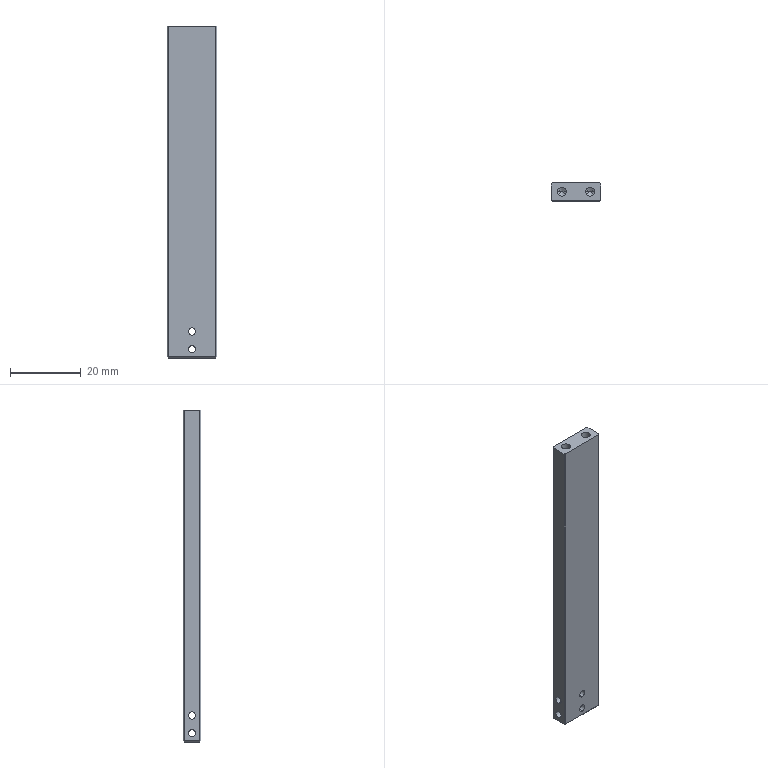Part | STEP file | Stopper bar | 1 solid | 42 faces | box 14 x 5 x 94 mm | volume 6342 mm3 | cylinder 20 | plane 18 | cone 4 | commonest cylinder face diameters 2.05 x16 2.5 x4